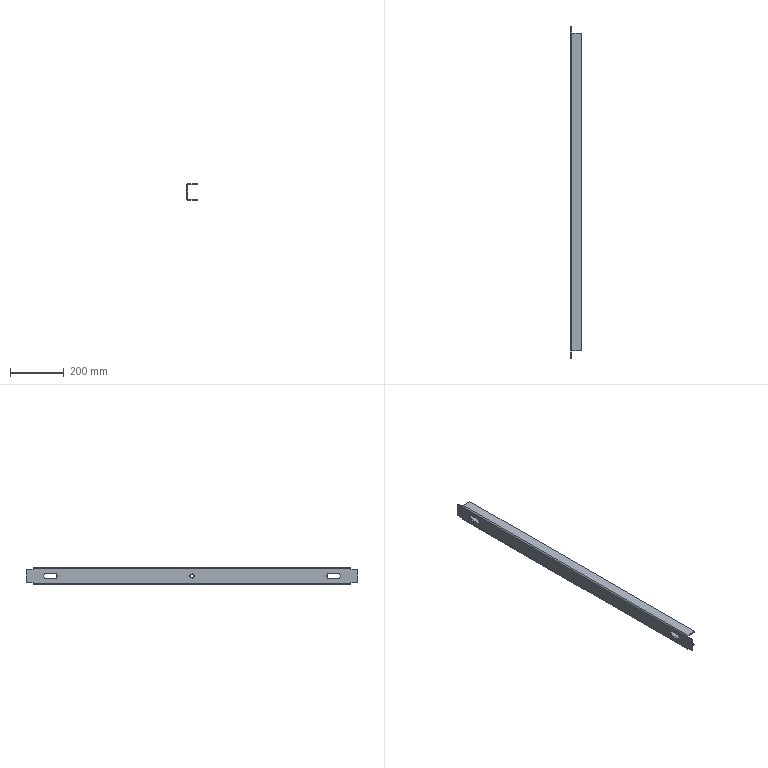Part | 1 solid | 44 faces | box 40 x 1230 x 62 mm | volume 624803 mm3 | plane 30 | cylinder 14 | commonest cylinder face diameters 10 x4 20 x4 0.4 x2 8.4 x2 15 x2
STEP:
#1=CARTESIAN_POINT('',(0.,0.,-7.5));
#2=VERTEX_POINT('',#1);
#3=CARTESIAN_POINT('',(0.,0.,7.5));
#4=VERTEX_POINT('',#3);
#5=CARTESIAN_POINT('',(0.,0.,0.));
#6=DIRECTION('',(-1.,0.,0.));
#7=DIRECTION('',(0.,0.,1.));
#8=AXIS2_PLACEMENT_3D('',#5,#6,#7);
#9=CIRCLE('',#8,7.5);
#10=EDGE_CURVE('',#2,#4,#9,.T.);
#11=ORIENTED_EDGE('',*,*,#10,.T.);
#12=CARTESIAN_POINT('',(4.,0.,7.5));
#13=VERTEX_POINT('',#12);
#14=CARTESIAN_POINT('',(-6.,0.,7.5));
#15=DIRECTION('',(1.,0.,0.));
#16=VECTOR('',#15,1000.);
#17=LINE('',#14,#16);
#18=EDGE_CURVE('',#4,#13,#17,.T.);
#19=ORIENTED_EDGE('',*,*,#18,.T.);
#20=CARTESIAN_POINT('',(4.,0.,-7.5));
#21=VERTEX_POINT('',#20);
#22=CARTESIAN_POINT('',(4.,0.,0.));
#23=DIRECTION('',(1.,0.,0.));
#24=DIRECTION('',(0.,0.,-1.));
#25=AXIS2_PLACEMENT_3D('',#22,#23,#24);
#26=CIRCLE('',#25,7.5);
#27=EDGE_CURVE('',#13,#21,#26,.T.);
#28=ORIENTED_EDGE('',*,*,#27,.T.);
#29=CARTESIAN_POINT('',(-6.,0.,-7.5));
#30=DIRECTION('',(1.,0.,0.));
#31=VECTOR('',#30,1000.);
#32=LINE('',#29,#31);
#33=EDGE_CURVE('',#2,#21,#32,.T.);
#34=ORIENTED_EDGE('',*,*,#33,.F.);
#35=EDGE_LOOP('',(#11,#19,#28,#34));
#36=FACE_OUTER_BOUND('',#35,.T.);
#37=CARTESIAN_POINT('',(-6.,0.,0.));
#38=DIRECTION('',(1.,0.,0.));
#39=DIRECTION('',(0.,0.,-1.));
#40=AXIS2_PLACEMENT_3D('',#37,#38,#39);
#41=CYLINDRICAL_SURFACE('',#40,7.5);
#42=ADVANCED_FACE('',(#36),#41,.F.);
#43=CARTESIAN_POINT('',(4.,-589.,25.));
#44=VERTEX_POINT('',#43);
#45=CARTESIAN_POINT('',(0.,-589.,25.));
#46=VERTEX_POINT('',#45);
#47=CARTESIAN_POINT('',(4.2,-589.,25.));
#48=DIRECTION('',(-1.,0.,0.));
#49=VECTOR('',#48,1000.);
#50=LINE('',#47,#49);
#51=EDGE_CURVE('',#44,#46,#50,.T.);
#52=ORIENTED_EDGE('',*,*,#51,.F.);
#53=CARTESIAN_POINT('',(4.,-589.,26.8));
#54=VERTEX_POINT('',#53);
#55=CARTESIAN_POINT('',(4.,-589.,-31.));
#56=DIRECTION('',(0.,0.,-1.));
#57=VECTOR('',#56,1000.);
#58=LINE('',#55,#57);
#59=EDGE_CURVE('',#54,#44,#58,.T.);
#60=ORIENTED_EDGE('',*,*,#59,.F.);
#61=CARTESIAN_POINT('',(0.,-589.,26.8));
#62=VERTEX_POINT('',#61);
#63=CARTESIAN_POINT('',(4.,-589.,26.8));
#64=DIRECTION('',(-1.,0.,0.));
#65=VECTOR('',#64,1000.);
#66=LINE('',#63,#65);
#67=EDGE_CURVE('',#54,#62,#66,.T.);
#68=ORIENTED_EDGE('',*,*,#67,.T.);
#69=CARTESIAN_POINT('',(0.,-589.,-31.));
#70=DIRECTION('',(0.,0.,-1.));
#71=VECTOR('',#70,1000.);
#72=LINE('',#69,#71);
#73=EDGE_CURVE('',#62,#46,#72,.T.);
#74=ORIENTED_EDGE('',*,*,#73,.T.);
#75=EDGE_LOOP('',(#52,#60,#68,#74));
#76=FACE_OUTER_BOUND('',#75,.T.);
#77=CARTESIAN_POINT('',(4.2,-589.,-27.));
#78=DIRECTION('',(0.,-1.,0.));
#79=DIRECTION('',(0.,0.,-1.));
#80=AXIS2_PLACEMENT_3D('',#77,#78,#79);
#81=PLANE('',#80);
#82=ADVANCED_FACE('',(#76),#81,.T.);
#83=CARTESIAN_POINT('',(4.,589.,-25.));
#84=VERTEX_POINT('',#83);
#85=CARTESIAN_POINT('',(0.,589.,-25.));
#86=VERTEX_POINT('',#85);
#87=CARTESIAN_POINT('',(4.2,589.,-25.));
#88=DIRECTION('',(-1.,0.,0.));
#89=VECTOR('',#88,1000.);
#90=LINE('',#87,#89);
#91=EDGE_CURVE('',#84,#86,#90,.T.);
#92=ORIENTED_EDGE('',*,*,#91,.F.);
#93=CARTESIAN_POINT('',(4.,589.,-26.8));
#94=VERTEX_POINT('',#93);
#95=CARTESIAN_POINT('',(4.,589.,-31.));
#96=DIRECTION('',(0.,0.,-1.));
#97=VECTOR('',#96,1000.);
#98=LINE('',#95,#97);
#99=EDGE_CURVE('',#84,#94,#98,.T.);
#100=ORIENTED_EDGE('',*,*,#99,.T.);
#101=CARTESIAN_POINT('',(0.,589.,-26.8));
#102=VERTEX_POINT('',#101);
#103=CARTESIAN_POINT('',(4.,589.,-26.8));
#104=DIRECTION('',(-1.,0.,0.));
#105=VECTOR('',#104,1000.);
#106=LINE('',#103,#105);
#107=EDGE_CURVE('',#94,#102,#106,.T.);
#108=ORIENTED_EDGE('',*,*,#107,.T.);
#109=CARTESIAN_POINT('',(0.,589.,-31.));
#110=DIRECTION('',(0.,0.,-1.));
#111=VECTOR('',#110,1000.);
#112=LINE('',#109,#111);
#113=EDGE_CURVE('',#86,#102,#112,.T.);
#114=ORIENTED_EDGE('',*,*,#113,.F.);
#115=EDGE_LOOP('',(#92,#100,#108,#114));
#116=FACE_OUTER_BOUND('',#115,.T.);
#117=CARTESIAN_POINT('',(4.2,589.,27.));
#118=DIRECTION('',(0.,1.,0.));
#119=DIRECTION('',(0.,0.,1.));
#120=AXIS2_PLACEMENT_3D('',#117,#118,#119);
#121=PLANE('',#120);
#122=ADVANCED_FACE('',(#116),#121,.T.);
#123=CARTESIAN_POINT('',(0.,589.,26.8));
#124=VERTEX_POINT('',#123);
#125=CARTESIAN_POINT('',(4.,589.,26.8));
#126=VERTEX_POINT('',#125);
#127=CARTESIAN_POINT('',(0.,589.,26.8));
#128=DIRECTION('',(1.,0.,0.));
#129=VECTOR('',#128,1000.);
#130=LINE('',#127,#129);
#131=EDGE_CURVE('',#124,#126,#130,.T.);
#132=ORIENTED_EDGE('',*,*,#131,.F.);
#133=CARTESIAN_POINT('',(4.2,589.,31.));
#134=VERTEX_POINT('',#133);
#135=CARTESIAN_POINT('',(4.2,589.,26.8));
#136=DIRECTION('',(0.,-1.,0.));
#137=DIRECTION('',(0.,0.,1.));
#138=AXIS2_PLACEMENT_3D('',#135,#136,#137);
#139=CIRCLE('',#138,4.2);
#140=EDGE_CURVE('',#134,#124,#139,.T.);
#141=ORIENTED_EDGE('',*,*,#140,.F.);
#142=CARTESIAN_POINT('',(4.2,589.,27.));
#143=VERTEX_POINT('',#142);
#144=CARTESIAN_POINT('',(4.2,589.,27.));
#145=DIRECTION('',(0.,0.,1.));
#146=VECTOR('',#145,1000.);
#147=LINE('',#144,#146);
#148=EDGE_CURVE('',#143,#134,#147,.T.);
#149=ORIENTED_EDGE('',*,*,#148,.F.);
#150=CARTESIAN_POINT('',(4.2,589.,26.8));
#151=DIRECTION('',(0.,-1.,0.));
#152=DIRECTION('',(1.,0.,0.));
#153=AXIS2_PLACEMENT_3D('',#150,#151,#152);
#154=CIRCLE('',#153,0.2);
#155=EDGE_CURVE('',#143,#126,#154,.T.);
#156=ORIENTED_EDGE('',*,*,#155,.T.);
#157=EDGE_LOOP('',(#132,#141,#149,#156));
#158=FACE_OUTER_BOUND('',#157,.T.);
#159=CARTESIAN_POINT('',(0.,589.,26.8));
#160=DIRECTION('',(0.,1.,0.));
#161=DIRECTION('',(0.,0.,1.));
#162=AXIS2_PLACEMENT_3D('',#159,#160,#161);
#163=PLANE('',#162);
#164=ADVANCED_FACE('',(#158),#163,.T.);
#165=CARTESIAN_POINT('',(0.,589.,25.));
#166=VERTEX_POINT('',#165);
#167=CARTESIAN_POINT('',(4.,589.,25.));
#168=VERTEX_POINT('',#167);
#169=CARTESIAN_POINT('',(4.2,589.,25.));
#170=DIRECTION('',(1.,0.,0.));
#171=VECTOR('',#170,1000.);
#172=LINE('',#169,#171);
#173=EDGE_CURVE('',#166,#168,#172,.T.);
#174=ORIENTED_EDGE('',*,*,#173,.F.);
#175=CARTESIAN_POINT('',(0.,589.,-31.));
#176=DIRECTION('',(0.,0.,-1.));
#177=VECTOR('',#176,1000.);
#178=LINE('',#175,#177);
#179=EDGE_CURVE('',#124,#166,#178,.T.);
#180=ORIENTED_EDGE('',*,*,#179,.F.);
#181=ORIENTED_EDGE('',*,*,#131,.T.);
#182=CARTESIAN_POINT('',(4.,589.,-31.));
#183=DIRECTION('',(0.,0.,-1.));
#184=VECTOR('',#183,1000.);
#185=LINE('',#182,#184);
#186=EDGE_CURVE('',#126,#168,#185,.T.);
#187=ORIENTED_EDGE('',*,*,#186,.T.);
#188=EDGE_LOOP('',(#174,#180,#181,#187));
#189=FACE_OUTER_BOUND('',#188,.T.);
#190=CARTESIAN_POINT('',(4.2,589.,27.));
#191=DIRECTION('',(0.,1.,0.));
#192=DIRECTION('',(0.,0.,1.));
#193=AXIS2_PLACEMENT_3D('',#190,#191,#192);
#194=PLANE('',#193);
#195=ADVANCED_FACE('',(#189),#194,.T.);
#196=CARTESIAN_POINT('',(4.2,-589.,31.));
#197=VERTEX_POINT('',#196);
#198=CARTESIAN_POINT('',(4.2,-589.,27.));
#199=VERTEX_POINT('',#198);
#200=CARTESIAN_POINT('',(4.2,-589.,31.));
#201=DIRECTION('',(0.,0.,-1.));
#202=VECTOR('',#201,1000.);
#203=LINE('',#200,#202);
#204=EDGE_CURVE('',#197,#199,#203,.T.);
#205=ORIENTED_EDGE('',*,*,#204,.F.);
#206=CARTESIAN_POINT('',(4.2,-589.,26.8));
#207=DIRECTION('',(0.,-1.,0.));
#208=DIRECTION('',(0.,0.,1.));
#209=AXIS2_PLACEMENT_3D('',#206,#207,#208);
#210=CIRCLE('',#209,4.2);
#211=EDGE_CURVE('',#197,#62,#210,.T.);
#212=ORIENTED_EDGE('',*,*,#211,.T.);
#213=ORIENTED_EDGE('',*,*,#67,.F.);
#214=CARTESIAN_POINT('',(4.2,-589.,26.8));
#215=DIRECTION('',(0.,-1.,0.));
#216=DIRECTION('',(1.,0.,0.));
#217=AXIS2_PLACEMENT_3D('',#214,#215,#216);
#218=CIRCLE('',#217,0.2);
#219=EDGE_CURVE('',#199,#54,#218,.T.);
#220=ORIENTED_EDGE('',*,*,#219,.F.);
#221=EDGE_LOOP('',(#205,#212,#213,#220));
#222=FACE_OUTER_BOUND('',#221,.T.);
#223=CARTESIAN_POINT('',(4.2,-589.,31.));
#224=DIRECTION('',(0.,-1.,0.));
#225=DIRECTION('',(0.,0.,-1.));
#226=AXIS2_PLACEMENT_3D('',#223,#224,#225);
#227=PLANE('',#226);
#228=ADVANCED_FACE('',(#222),#227,.T.);
#229=CARTESIAN_POINT('',(40.,-589.,31.));
#230=VERTEX_POINT('',#229);
#231=CARTESIAN_POINT('',(0.,-589.,31.));
#232=DIRECTION('',(-1.,0.,0.));
#233=VECTOR('',#232,1000.);
#234=LINE('',#231,#233);
#235=EDGE_CURVE('',#230,#197,#234,.T.);
#236=ORIENTED_EDGE('',*,*,#235,.T.);
#237=ORIENTED_EDGE('',*,*,#204,.T.);
#238=CARTESIAN_POINT('',(40.,-589.,27.));
#239=VERTEX_POINT('',#238);
#240=CARTESIAN_POINT('',(0.,-589.,27.));
#241=DIRECTION('',(-1.,0.,0.));
#242=VECTOR('',#241,1000.);
#243=LINE('',#240,#242);
#244=EDGE_CURVE('',#239,#199,#243,.T.);
#245=ORIENTED_EDGE('',*,*,#244,.F.);
#246=CARTESIAN_POINT('',(40.,-589.,27.));
#247=DIRECTION('',(0.,0.,1.));
#248=VECTOR('',#247,1000.);
#249=LINE('',#246,#248);
#250=EDGE_CURVE('',#239,#230,#249,.T.);
#251=ORIENTED_EDGE('',*,*,#250,.T.);
#252=EDGE_LOOP('',(#236,#237,#245,#251));
#253=FACE_OUTER_BOUND('',#252,.T.);
#254=CARTESIAN_POINT('',(4.,-589.,26.8));
#255=DIRECTION('',(0.,-1.,0.));
#256=DIRECTION('',(0.,0.,-1.));
#257=AXIS2_PLACEMENT_3D('',#254,#255,#256);
#258=PLANE('',#257);
#259=ADVANCED_FACE('',(#253),#258,.T.);
#260=CARTESIAN_POINT('',(4.2,589.,-31.));
#261=VERTEX_POINT('',#260);
#262=CARTESIAN_POINT('',(4.2,589.,-27.));
#263=VERTEX_POINT('',#262);
#264=CARTESIAN_POINT('',(4.2,589.,-31.));
#265=DIRECTION('',(0.,0.,1.));
#266=VECTOR('',#265,1000.);
#267=LINE('',#264,#266);
#268=EDGE_CURVE('',#261,#263,#267,.T.);
#269=ORIENTED_EDGE('',*,*,#268,.F.);
#270=CARTESIAN_POINT('',(4.2,589.,-26.8));
#271=DIRECTION('',(0.,-1.,0.));
#272=DIRECTION('',(0.,0.,1.));
#273=AXIS2_PLACEMENT_3D('',#270,#271,#272);
#274=CIRCLE('',#273,4.2);
#275=EDGE_CURVE('',#102,#261,#274,.T.);
#276=ORIENTED_EDGE('',*,*,#275,.F.);
#277=ORIENTED_EDGE('',*,*,#107,.F.);
#278=CARTESIAN_POINT('',(4.2,589.,-26.8));
#279=DIRECTION('',(0.,-1.,0.));
#280=DIRECTION('',(1.,0.,0.));
#281=AXIS2_PLACEMENT_3D('',#278,#279,#280);
#282=CIRCLE('',#281,0.2);
#283=EDGE_CURVE('',#94,#263,#282,.T.);
#284=ORIENTED_EDGE('',*,*,#283,.T.);
#285=EDGE_LOOP('',(#269,#276,#277,#284));
#286=FACE_OUTER_BOUND('',#285,.T.);
#287=CARTESIAN_POINT('',(4.2,589.,-31.));
#288=DIRECTION('',(0.,1.,0.));
#289=DIRECTION('',(0.,0.,1.));
#290=AXIS2_PLACEMENT_3D('',#287,#288,#289);
#291=PLANE('',#290);
#292=ADVANCED_FACE('',(#286),#291,.T.);
#293=CARTESIAN_POINT('',(40.,589.,-31.));
#294=VERTEX_POINT('',#293);
#295=CARTESIAN_POINT('',(0.,589.,-31.));
#296=DIRECTION('',(1.,0.,0.));
#297=VECTOR('',#296,1000.);
#298=LINE('',#295,#297);
#299=EDGE_CURVE('',#261,#294,#298,.T.);
#300=ORIENTED_EDGE('',*,*,#299,.F.);
#301=ORIENTED_EDGE('',*,*,#268,.T.);
#302=CARTESIAN_POINT('',(40.,589.,-27.));
#303=VERTEX_POINT('',#302);
#304=CARTESIAN_POINT('',(0.,589.,-27.));
#305=DIRECTION('',(1.,0.,0.));
#306=VECTOR('',#305,1000.);
#307=LINE('',#304,#306);
#308=EDGE_CURVE('',#263,#303,#307,.T.);
#309=ORIENTED_EDGE('',*,*,#308,.T.);
#310=CARTESIAN_POINT('',(40.,589.,-31.));
#311=DIRECTION('',(0.,0.,1.));
#312=VECTOR('',#311,1000.);
#313=LINE('',#310,#312);
#314=EDGE_CURVE('',#294,#303,#313,.T.);
#315=ORIENTED_EDGE('',*,*,#314,.F.);
#316=EDGE_LOOP('',(#300,#301,#309,#315));
#317=FACE_OUTER_BOUND('',#316,.T.);
#318=CARTESIAN_POINT('',(4.,589.,-26.8));
#319=DIRECTION('',(0.,1.,0.));
#320=DIRECTION('',(0.,0.,1.));
#321=AXIS2_PLACEMENT_3D('',#318,#319,#320);
#322=PLANE('',#321);
#323=ADVANCED_FACE('',(#317),#322,.T.);
#324=CARTESIAN_POINT('',(0.,-589.,-26.8));
#325=VERTEX_POINT('',#324);
#326=CARTESIAN_POINT('',(4.,-589.,-26.8));
#327=VERTEX_POINT('',#326);
#328=CARTESIAN_POINT('',(0.,-589.,-26.8));
#329=DIRECTION('',(1.,0.,0.));
#330=VECTOR('',#329,1000.);
#331=LINE('',#328,#330);
#332=EDGE_CURVE('',#325,#327,#331,.T.);
#333=ORIENTED_EDGE('',*,*,#332,.F.);
#334=CARTESIAN_POINT('',(4.2,-589.,-31.));
#335=VERTEX_POINT('',#334);
#336=CARTESIAN_POINT('',(4.2,-589.,-26.8));
#337=DIRECTION('',(0.,-1.,0.));
#338=DIRECTION('',(0.,0.,1.));
#339=AXIS2_PLACEMENT_3D('',#336,#337,#338);
#340=CIRCLE('',#339,4.2);
#341=EDGE_CURVE('',#325,#335,#340,.T.);
#342=ORIENTED_EDGE('',*,*,#341,.T.);
#343=CARTESIAN_POINT('',(4.2,-589.,-27.));
#344=VERTEX_POINT('',#343);
#345=CARTESIAN_POINT('',(4.2,-589.,-27.));
#346=DIRECTION('',(0.,0.,-1.));
#347=VECTOR('',#346,1000.);
#348=LINE('',#345,#347);
#349=EDGE_CURVE('',#344,#335,#348,.T.);
#350=ORIENTED_EDGE('',*,*,#349,.F.);
#351=CARTESIAN_POINT('',(4.2,-589.,-26.8));
#352=DIRECTION('',(0.,-1.,0.));
#353=DIRECTION('',(1.,0.,0.));
#354=AXIS2_PLACEMENT_3D('',#351,#352,#353);
#355=CIRCLE('',#354,0.2);
#356=EDGE_CURVE('',#327,#344,#355,.T.);
#357=ORIENTED_EDGE('',*,*,#356,.F.);
#358=EDGE_LOOP('',(#333,#342,#350,#357));
#359=FACE_OUTER_BOUND('',#358,.T.);
#360=CARTESIAN_POINT('',(0.,-589.,-26.8));
#361=DIRECTION('',(0.,-1.,0.));
#362=DIRECTION('',(0.,0.,-1.));
#363=AXIS2_PLACEMENT_3D('',#360,#361,#362);
#364=PLANE('',#363);
#365=ADVANCED_FACE('',(#359),#364,.T.);
#366=CARTESIAN_POINT('',(0.,-589.,-25.));
#367=VERTEX_POINT('',#366);
#368=CARTESIAN_POINT('',(4.,-589.,-25.));
#369=VERTEX_POINT('',#368);
#370=CARTESIAN_POINT('',(4.2,-589.,-25.));
#371=DIRECTION('',(1.,0.,0.));
#372=VECTOR('',#371,1000.);
#373=LINE('',#370,#372);
#374=EDGE_CURVE('',#367,#369,#373,.T.);
#375=ORIENTED_EDGE('',*,*,#374,.F.);
#376=CARTESIAN_POINT('',(0.,-589.,-31.));
#377=DIRECTION('',(0.,0.,-1.));
#378=VECTOR('',#377,1000.);
#379=LINE('',#376,#378);
#380=EDGE_CURVE('',#367,#325,#379,.T.);
#381=ORIENTED_EDGE('',*,*,#380,.T.);
#382=ORIENTED_EDGE('',*,*,#332,.T.);
#383=CARTESIAN_POINT('',(4.,-589.,-31.));
#384=DIRECTION('',(0.,0.,-1.));
#385=VECTOR('',#384,1000.);
#386=LINE('',#383,#385);
#387=EDGE_CURVE('',#369,#327,#386,.T.);
#388=ORIENTED_EDGE('',*,*,#387,.F.);
#389=EDGE_LOOP('',(#375,#381,#382,#388));
#390=FACE_OUTER_BOUND('',#389,.T.);
#391=CARTESIAN_POINT('',(4.2,-589.,-27.));
#392=DIRECTION('',(0.,-1.,0.));
#393=DIRECTION('',(0.,0.,-1.));
#394=AXIS2_PLACEMENT_3D('',#391,#392,#393);
#395=PLANE('',#394);
#396=ADVANCED_FACE('',(#390),#395,.T.);
#397=CARTESIAN_POINT('',(40.,-589.,-27.));
#398=VERTEX_POINT('',#397);
#399=CARTESIAN_POINT('',(0.,-589.,-27.));
#400=DIRECTION('',(1.,0.,0.));
#401=VECTOR('',#400,1000.);
#402=LINE('',#399,#401);
#403=EDGE_CURVE('',#344,#398,#402,.T.);
#404=ORIENTED_EDGE('',*,*,#403,.T.);
#405=CARTESIAN_POINT('',(40.,589.,-27.));
#406=DIRECTION('',(0.,-1.,0.));
#407=VECTOR('',#406,1000.);
#408=LINE('',#405,#407);
#409=EDGE_CURVE('',#303,#398,#408,.T.);
#410=ORIENTED_EDGE('',*,*,#409,.F.);
#411=ORIENTED_EDGE('',*,*,#308,.F.);
#412=CARTESIAN_POINT('',(4.2,589.,-27.));
#413=DIRECTION('',(0.,-1.,0.));
#414=VECTOR('',#413,1000.);
#415=LINE('',#412,#414);
#416=EDGE_CURVE('',#263,#344,#415,.T.);
#417=ORIENTED_EDGE('',*,*,#416,.T.);
#418=EDGE_LOOP('',(#404,#410,#411,#417));
#419=FACE_OUTER_BOUND('',#418,.T.);
#420=CARTESIAN_POINT('',(0.,589.,-27.));
#421=DIRECTION('',(0.,0.,-1.));
#422=DIRECTION('',(-1.,0.,0.));
#423=AXIS2_PLACEMENT_3D('',#420,#421,#422);
#424=PLANE('',#423);
#425=ADVANCED_FACE('',(#419),#424,.F.);
#426=CARTESIAN_POINT('',(40.,-589.,-31.));
#427=VERTEX_POINT('',#426);
#428=CARTESIAN_POINT('',(40.,-589.,-31.));
#429=DIRECTION('',(0.,0.,1.));
#430=VECTOR('',#429,1000.);
#431=LINE('',#428,#430);
#432=EDGE_CURVE('',#427,#398,#431,.T.);
#433=ORIENTED_EDGE('',*,*,#432,.F.);
#434=CARTESIAN_POINT('',(40.,589.,-31.));
#435=DIRECTION('',(0.,-1.,0.));
#436=VECTOR('',#435,1000.);
#437=LINE('',#434,#436);
#438=EDGE_CURVE('',#294,#427,#437,.T.);
#439=ORIENTED_EDGE('',*,*,#438,.F.);
#440=ORIENTED_EDGE('',*,*,#314,.T.);
#441=ORIENTED_EDGE('',*,*,#409,.T.);
#442=EDGE_LOOP('',(#433,#439,#440,#441));
#443=FACE_OUTER_BOUND('',#442,.T.);
#444=CARTESIAN_POINT('',(40.,589.,-31.));
#445=DIRECTION('',(1.,0.,0.));
#446=DIRECTION('',(0.,0.,-1.));
#447=AXIS2_PLACEMENT_3D('',#444,#445,#446);
#448=PLANE('',#447);
#449=ADVANCED_FACE('',(#443),#448,.T.);
#450=CARTESIAN_POINT('',(0.,-589.,-31.));
#451=DIRECTION('',(1.,0.,0.));
#452=VECTOR('',#451,1000.);
#453=LINE('',#450,#452);
#454=EDGE_CURVE('',#335,#427,#453,.T.);
#455=ORIENTED_EDGE('',*,*,#454,.F.);
#456=CARTESIAN_POINT('',(4.2,589.,-31.));
#457=DIRECTION('',(0.,-1.,0.));
#458=VECTOR('',#457,1000.);
#459=LINE('',#456,#458);
#460=EDGE_CURVE('',#261,#335,#459,.T.);
#461=ORIENTED_EDGE('',*,*,#460,.F.);
#462=ORIENTED_EDGE('',*,*,#299,.T.);
#463=ORIENTED_EDGE('',*,*,#438,.T.);
#464=EDGE_LOOP('',(#455,#461,#462,#463));
#465=FACE_OUTER_BOUND('',#464,.T.);
#466=CARTESIAN_POINT('',(0.,589.,-31.));
#467=DIRECTION('',(0.,0.,-1.));
#468=DIRECTION('',(-1.,0.,0.));
#469=AXIS2_PLACEMENT_3D('',#466,#467,#468);
#470=PLANE('',#469);
#471=ADVANCED_FACE('',(#465),#470,.T.);
#472=ORIENTED_EDGE('',*,*,#341,.F.);
#473=CARTESIAN_POINT('',(0.,589.,-26.8));
#474=DIRECTION('',(0.,-1.,0.));
#475=VECTOR('',#474,1000.);
#476=LINE('',#473,#475);
#477=EDGE_CURVE('',#102,#325,#476,.T.);
#478=ORIENTED_EDGE('',*,*,#477,.F.);
#479=ORIENTED_EDGE('',*,*,#275,.T.);
#480=ORIENTED_EDGE('',*,*,#460,.T.);
#481=EDGE_LOOP('',(#472,#478,#479,#480));
#482=FACE_OUTER_BOUND('',#481,.T.);
#483=CARTESIAN_POINT('',(4.2,589.,-26.8));
#484=DIRECTION('',(0.,-1.,0.));
#485=DIRECTION('',(0.,0.,-1.));
#486=AXIS2_PLACEMENT_3D('',#483,#484,#485);
#487=CYLINDRICAL_SURFACE('',#486,4.2);
#488=ADVANCED_FACE('',(#482),#487,.T.);
#489=CARTESIAN_POINT('',(0.,510.,-10.));
#490=VERTEX_POINT('',#489);
#491=CARTESIAN_POINT('',(0.,510.,10.));
#492=VERTEX_POINT('',#491);
#493=CARTESIAN_POINT('',(0.,510.,0.));
#494=DIRECTION('',(-1.,0.,0.));
#495=DIRECTION('',(0.,0.,1.));
#496=AXIS2_PLACEMENT_3D('',#493,#494,#495);
#497=CIRCLE('',#496,10.);
#498=EDGE_CURVE('',#490,#492,#497,.T.);
#499=ORIENTED_EDGE('',*,*,#498,.F.);
#500=CARTESIAN_POINT('',(0.,540.,-10.));
#501=VERTEX_POINT('',#500);
#502=CARTESIAN_POINT('',(0.,589.,-10.));
#503=DIRECTION('',(0.,-1.,0.));
#504=VECTOR('',#503,1000.);
#505=LINE('',#502,#504);
#506=EDGE_CURVE('',#501,#490,#505,.T.);
#507=ORIENTED_EDGE('',*,*,#506,.F.);
#508=CARTESIAN_POINT('',(0.,540.,10.));
#509=VERTEX_POINT('',#508);
#510=CARTESIAN_POINT('',(0.,540.,0.));
#511=DIRECTION('',(-1.,0.,0.));
#512=DIRECTION('',(0.,0.,1.));
#513=AXIS2_PLACEMENT_3D('',#510,#511,#512);
#514=CIRCLE('',#513,10.);
#515=EDGE_CURVE('',#509,#501,#514,.T.);
#516=ORIENTED_EDGE('',*,*,#515,.F.);
#517=CARTESIAN_POINT('',(0.,589.,10.));
#518=DIRECTION('',(0.,1.,0.));
#519=VECTOR('',#518,1000.);
#520=LINE('',#517,#519);
#521=EDGE_CURVE('',#492,#509,#520,.T.);
#522=ORIENTED_EDGE('',*,*,#521,.F.);
#523=EDGE_LOOP('',(#499,#507,#516,#522));
#524=FACE_BOUND('',#523,.T.);
#525=ORIENTED_EDGE('',*,*,#10,.F.);
#526=CARTESIAN_POINT('',(0.,0.,0.));
#527=DIRECTION('',(-1.,0.,0.));
#528=DIRECTION('',(0.,0.,1.));
#529=AXIS2_PLACEMENT_3D('',#526,#527,#528);
#530=CIRCLE('',#529,7.5);
#531=EDGE_CURVE('',#4,#2,#530,.T.);
#532=ORIENTED_EDGE('',*,*,#531,.F.);
#533=EDGE_LOOP('',(#525,#532));
#534=FACE_BOUND('',#533,.T.);
#535=CARTESIAN_POINT('',(0.,-510.,10.));
#536=VERTEX_POINT('',#535);
#537=CARTESIAN_POINT('',(0.,-510.,-10.));
#538=VERTEX_POINT('',#537);
#539=CARTESIAN_POINT('',(0.,-510.,0.));
#540=DIRECTION('',(-1.,0.,0.));
#541=DIRECTION('',(0.,0.,1.));
#542=AXIS2_PLACEMENT_3D('',#539,#540,#541);
#543=CIRCLE('',#542,10.);
#544=EDGE_CURVE('',#536,#538,#543,.T.);
#545=ORIENTED_EDGE('',*,*,#544,.F.);
#546=CARTESIAN_POINT('',(0.,-540.,10.));
#547=VERTEX_POINT('',#546);
#548=CARTESIAN_POINT('',(0.,589.,10.));
#549=DIRECTION('',(0.,1.,0.));
#550=VECTOR('',#549,1000.);
#551=LINE('',#548,#550);
#552=EDGE_CURVE('',#547,#536,#551,.T.);
#553=ORIENTED_EDGE('',*,*,#552,.F.);
#554=CARTESIAN_POINT('',(0.,-540.,-10.));
#555=VERTEX_POINT('',#554);
#556=CARTESIAN_POINT('',(0.,-540.,0.));
#557=DIRECTION('',(-1.,0.,0.));
#558=DIRECTION('',(0.,0.,1.));
#559=AXIS2_PLACEMENT_3D('',#556,#557,#558);
#560=CIRCLE('',#559,10.);
#561=EDGE_CURVE('',#555,#547,#560,.T.);
#562=ORIENTED_EDGE('',*,*,#561,.F.);
#563=CARTESIAN_POINT('',(0.,589.,-10.));
#564=DIRECTION('',(0.,-1.,0.));
#565=VECTOR('',#564,1000.);
#566=LINE('',#563,#565);
#567=EDGE_CURVE('',#538,#555,#566,.T.);
#568=ORIENTED_EDGE('',*,*,#567,.F.);
#569=EDGE_LOOP('',(#545,#553,#562,#568));
#570=FACE_BOUND('',#569,.T.);
#571=CARTESIAN_POINT('',(0.,-610.,-25.));
#572=VERTEX_POINT('',#571);
#573=CARTESIAN_POINT('',(0.,-615.,-25.));
#574=DIRECTION('',(0.,1.,0.));
#575=VECTOR('',#574,1000.);
#576=LINE('',#573,#575);
#577=EDGE_CURVE('',#572,#367,#576,.T.);
#578=ORIENTED_EDGE('',*,*,#577,.F.);
#579=CARTESIAN_POINT('',(0.,-615.,-20.));
#580=VERTEX_POINT('',#579);
#581=CARTESIAN_POINT('',(0.,-610.,-20.));
#582=DIRECTION('',(-1.,0.,0.));
#583=DIRECTION('',(0.,0.,1.));
#584=AXIS2_PLACEMENT_3D('',#581,#582,#583);
#585=CIRCLE('',#584,5.);
#586=EDGE_CURVE('',#572,#580,#585,.T.);
#587=ORIENTED_EDGE('',*,*,#586,.T.);
#588=CARTESIAN_POINT('',(0.,-615.,20.));
#589=VERTEX_POINT('',#588);
#590=CARTESIAN_POINT('',(0.,-615.,25.));
#591=DIRECTION('',(0.,0.,-1.));
#592=VECTOR('',#591,1000.);
#593=LINE('',#590,#592);
#594=EDGE_CURVE('',#589,#580,#593,.T.);
#595=ORIENTED_EDGE('',*,*,#594,.F.);
#596=CARTESIAN_POINT('',(0.,-610.,25.));
#597=VERTEX_POINT('',#596);
#598=CARTESIAN_POINT('',(0.,-610.,20.));
#599=DIRECTION('',(-1.,0.,0.));
#600=DIRECTION('',(0.,0.,1.));
#601=AXIS2_PLACEMENT_3D('',#598,#599,#600);
#602=CIRCLE('',#601,5.);
#603=EDGE_CURVE('',#589,#597,#602,.T.);
#604=ORIENTED_EDGE('',*,*,#603,.T.);
#605=CARTESIAN_POINT('',(0.,-615.,25.));
#606=DIRECTION('',(0.,-1.,0.));
#607=VECTOR('',#606,1000.);
#608=LINE('',#605,#607);
#609=EDGE_CURVE('',#46,#597,#608,.T.);
#610=ORIENTED_EDGE('',*,*,#609,.F.);
#611=ORIENTED_EDGE('',*,*,#73,.F.);
#612=CARTESIAN_POINT('',(0.,589.,26.8));
#613=DIRECTION('',(0.,-1.,0.));
#614=VECTOR('',#613,1000.);
#615=LINE('',#612,#614);
#616=EDGE_CURVE('',#124,#62,#615,.T.);
#617=ORIENTED_EDGE('',*,*,#616,.F.);
#618=ORIENTED_EDGE('',*,*,#179,.T.);
#619=CARTESIAN_POINT('',(0.,610.,25.));
#620=VERTEX_POINT('',#619);
#621=CARTESIAN_POINT('',(0.,615.,25.));
#622=DIRECTION('',(0.,-1.,0.));
#623=VECTOR('',#622,1000.);
#624=LINE('',#621,#623);
#625=EDGE_CURVE('',#620,#166,#624,.T.);
#626=ORIENTED_EDGE('',*,*,#625,.F.);
#627=CARTESIAN_POINT('',(0.,615.,20.));
#628=VERTEX_POINT('',#627);
#629=CARTESIAN_POINT('',(0.,610.,20.));
#630=DIRECTION('',(-1.,0.,0.));
#631=DIRECTION('',(0.,0.,1.));
#632=AXIS2_PLACEMENT_3D('',#629,#630,#631);
#633=CIRCLE('',#632,5.);
#634=EDGE_CURVE('',#620,#628,#633,.T.);
#635=ORIENTED_EDGE('',*,*,#634,.T.);
#636=CARTESIAN_POINT('',(0.,615.,-20.));
#637=VERTEX_POINT('',#636);
#638=CARTESIAN_POINT('',(0.,615.,25.));
#639=DIRECTION('',(0.,0.,1.));
#640=VECTOR('',#639,1000.);
#641=LINE('',#638,#640);
#642=EDGE_CURVE('',#637,#628,#641,.T.);
#643=ORIENTED_EDGE('',*,*,#642,.F.);
#644=CARTESIAN_POINT('',(0.,610.,-25.));
#645=VERTEX_POINT('',#644);
#646=CARTESIAN_POINT('',(0.,610.,-20.));
#647=DIRECTION('',(-1.,0.,0.));
#648=DIRECTION('',(0.,0.,1.));
#649=AXIS2_PLACEMENT_3D('',#646,#647,#648);
#650=CIRCLE('',#649,5.);
#651=EDGE_CURVE('',#637,#645,#650,.T.);
#652=ORIENTED_EDGE('',*,*,#651,.T.);
#653=CARTESIAN_POINT('',(0.,615.,-25.));
#654=DIRECTION('',(0.,1.,0.));
#655=VECTOR('',#654,1000.);
#656=LINE('',#653,#655);
#657=EDGE_CURVE('',#86,#645,#656,.T.);
#658=ORIENTED_EDGE('',*,*,#657,.F.);
#659=ORIENTED_EDGE('',*,*,#113,.T.);
#660=ORIENTED_EDGE('',*,*,#477,.T.);
#661=ORIENTED_EDGE('',*,*,#380,.F.);
#662=EDGE_LOOP('',(#578,#587,#595,#604,#610,#611,#617,#618,#626,#635,#643,#652,#658,#659,#660,#661));
#663=FACE_OUTER_BOUND('',#662,.T.);
#664=CARTESIAN_POINT('',(0.,589.,-31.));
#665=DIRECTION('',(-1.,0.,0.));
#666=DIRECTION('',(0.,0.,1.));
#667=AXIS2_PLACEMENT_3D('',#664,#665,#666);
#668=PLANE('',#667);
#669=ADVANCED_FACE('',(#524,#534,#570,#663),#668,.T.);
#670=ORIENTED_EDGE('',*,*,#211,.F.);
#671=CARTESIAN_POINT('',(4.2,589.,31.));
#672=DIRECTION('',(0.,-1.,0.));
#673=VECTOR('',#672,1000.);
#674=LINE('',#671,#673);
#675=EDGE_CURVE('',#134,#197,#674,.T.);
#676=ORIENTED_EDGE('',*,*,#675,.F.);
#677=ORIENTED_EDGE('',*,*,#140,.T.);
#678=ORIENTED_EDGE('',*,*,#616,.T.);
#679=EDGE_LOOP('',(#670,#676,#677,#678));
#680=FACE_OUTER_BOUND('',#679,.T.);
#681=CARTESIAN_POINT('',(4.2,589.,26.8));
#682=DIRECTION('',(0.,-1.,0.));
#683=DIRECTION('',(0.,0.,-1.));
#684=AXIS2_PLACEMENT_3D('',#681,#682,#683);
#685=CYLINDRICAL_SURFACE('',#684,4.2);
#686=ADVANCED_FACE('',(#680),#685,.T.);
#687=ORIENTED_EDGE('',*,*,#235,.F.);
#688=CARTESIAN_POINT('',(40.,589.,31.));
#689=VERTEX_POINT('',#688);
#690=CARTESIAN_POINT('',(40.,589.,31.));
#691=DIRECTION('',(0.,-1.,0.));
#692=VECTOR('',#691,1000.);
#693=LINE('',#690,#692);
#694=EDGE_CURVE('',#689,#230,#693,.T.);
#695=ORIENTED_EDGE('',*,*,#694,.F.);
#696=CARTESIAN_POINT('',(0.,589.,31.));
#697=DIRECTION('',(-1.,0.,0.));
#698=VECTOR('',#697,1000.);
#699=LINE('',#696,#698);
#700=EDGE_CURVE('',#689,#134,#699,.T.);
#701=ORIENTED_EDGE('',*,*,#700,.T.);
#702=ORIENTED_EDGE('',*,*,#675,.T.);
#703=EDGE_LOOP('',(#687,#695,#701,#702));
#704=FACE_OUTER_BOUND('',#703,.T.);
#705=CARTESIAN_POINT('',(0.,589.,31.));
#706=DIRECTION('',(0.,0.,1.));
#707=DIRECTION('',(1.,0.,0.));
#708=AXIS2_PLACEMENT_3D('',#705,#706,#707);
#709=PLANE('',#708);
#710=ADVANCED_FACE('',(#704),#709,.T.);
#711=ORIENTED_EDGE('',*,*,#250,.F.);
#712=CARTESIAN_POINT('',(40.,589.,27.));
#713=VERTEX_POINT('',#712);
#714=CARTESIAN_POINT('',(40.,589.,27.));
#715=DIRECTION('',(0.,-1.,0.));
#716=VECTOR('',#715,1000.);
#717=LINE('',#714,#716);
#718=EDGE_CURVE('',#713,#239,#717,.T.);
#719=ORIENTED_EDGE('',*,*,#718,.F.);
#720=CARTESIAN_POINT('',(40.,589.,27.));
#721=DIRECTION('',(0.,0.,1.));
#722=VECTOR('',#721,1000.);
#723=LINE('',#720,#722);
#724=EDGE_CURVE('',#713,#689,#723,.T.);
#725=ORIENTED_EDGE('',*,*,#724,.T.);
#726=ORIENTED_EDGE('',*,*,#694,.T.);
#727=EDGE_LOOP('',(#711,#719,#725,#726));
#728=FACE_OUTER_BOUND('',#727,.T.);
#729=CARTESIAN_POINT('',(40.,589.,27.));
#730=DIRECTION('',(1.,0.,0.));
#731=DIRECTION('',(0.,0.,-1.));
#732=AXIS2_PLACEMENT_3D('',#729,#730,#731);
#733=PLANE('',#732);
#734=ADVANCED_FACE('',(#728),#733,.T.);
#735=ORIENTED_EDGE('',*,*,#244,.T.);
#736=CARTESIAN_POINT('',(4.2,589.,27.));
#737=DIRECTION('',(0.,-1.,0.));
#738=VECTOR('',#737,1000.);
#739=LINE('',#736,#738);
#740=EDGE_CURVE('',#143,#199,#739,.T.);
#741=ORIENTED_EDGE('',*,*,#740,.F.);
#742=CARTESIAN_POINT('',(0.,589.,27.));
#743=DIRECTION('',(-1.,0.,0.));
#744=VECTOR('',#743,1000.);
#745=LINE('',#742,#744);
#746=EDGE_CURVE('',#713,#143,#745,.T.);
#747=ORIENTED_EDGE('',*,*,#746,.F.);
#748=ORIENTED_EDGE('',*,*,#718,.T.);
#749=EDGE_LOOP('',(#735,#741,#747,#748));
#750=FACE_OUTER_BOUND('',#749,.T.);
#751=CARTESIAN_POINT('',(0.,589.,27.));
#752=DIRECTION('',(0.,0.,1.));
#753=DIRECTION('',(1.,0.,0.));
#754=AXIS2_PLACEMENT_3D('',#751,#752,#753);
#755=PLANE('',#754);
#756=ADVANCED_FACE('',(#750),#755,.F.);
#757=ORIENTED_EDGE('',*,*,#219,.T.);
#758=CARTESIAN_POINT('',(4.,589.,26.8));
#759=DIRECTION('',(0.,-1.,0.));
#760=VECTOR('',#759,1000.);
#761=LINE('',#758,#760);
#762=EDGE_CURVE('',#126,#54,#761,.T.);
#763=ORIENTED_EDGE('',*,*,#762,.F.);
#764=ORIENTED_EDGE('',*,*,#155,.F.);
#765=ORIENTED_EDGE('',*,*,#740,.T.);
#766=EDGE_LOOP('',(#757,#763,#764,#765));
#767=FACE_OUTER_BOUND('',#766,.T.);
#768=CARTESIAN_POINT('',(4.2,589.,26.8));
#769=DIRECTION('',(0.,-1.,0.));
#770=DIRECTION('',(0.,0.,-1.));
#771=AXIS2_PLACEMENT_3D('',#768,#769,#770);
#772=CYLINDRICAL_SURFACE('',#771,0.2);
#773=ADVANCED_FACE('',(#767),#772,.F.);
#774=CARTESIAN_POINT('',(4.,510.,-10.));
#775=VERTEX_POINT('',#774);
#776=CARTESIAN_POINT('',(4.,540.,-10.));
#777=VERTEX_POINT('',#776);
#778=CARTESIAN_POINT('',(4.,510.,-10.));
#779=DIRECTION('',(0.,1.,0.));
#780=VECTOR('',#779,1000.);
#781=LINE('',#778,#780);
#782=EDGE_CURVE('',#775,#777,#781,.T.);
#783=ORIENTED_EDGE('',*,*,#782,.F.);
#784=CARTESIAN_POINT('',(4.,510.,10.));
#785=VERTEX_POINT('',#784);
#786=CARTESIAN_POINT('',(4.,510.,0.));
#787=DIRECTION('',(1.,0.,0.));
#788=DIRECTION('',(0.,0.,-1.));
#789=AXIS2_PLACEMENT_3D('',#786,#787,#788);
#790=CIRCLE('',#789,10.);
#791=EDGE_CURVE('',#785,#775,#790,.T.);
#792=ORIENTED_EDGE('',*,*,#791,.F.);
#793=CARTESIAN_POINT('',(4.,540.,10.));
#794=VERTEX_POINT('',#793);
#795=CARTESIAN_POINT('',(4.,510.,10.));
#796=DIRECTION('',(0.,-1.,0.));
#797=VECTOR('',#796,1000.);
#798=LINE('',#795,#797);
#799=EDGE_CURVE('',#794,#785,#798,.T.);
#800=ORIENTED_EDGE('',*,*,#799,.F.);
#801=CARTESIAN_POINT('',(4.,540.,0.));
#802=DIRECTION('',(1.,0.,0.));
#803=DIRECTION('',(0.,0.,-1.));
#804=AXIS2_PLACEMENT_3D('',#801,#802,#803);
#805=CIRCLE('',#804,10.);
#806=EDGE_CURVE('',#777,#794,#805,.T.);
#807=ORIENTED_EDGE('',*,*,#806,.F.);
#808=EDGE_LOOP('',(#783,#792,#800,#807));
#809=FACE_BOUND('',#808,.T.);
#810=CARTESIAN_POINT('',(4.,0.,0.));
#811=DIRECTION('',(1.,0.,0.));
#812=DIRECTION('',(0.,0.,-1.));
#813=AXIS2_PLACEMENT_3D('',#810,#811,#812);
#814=CIRCLE('',#813,7.5);
#815=EDGE_CURVE('',#21,#13,#814,.T.);
#816=ORIENTED_EDGE('',*,*,#815,.F.);
#817=ORIENTED_EDGE('',*,*,#27,.F.);
#818=EDGE_LOOP('',(#816,#817));
#819=FACE_BOUND('',#818,.T.);
#820=CARTESIAN_POINT('',(4.,-510.,10.));
#821=VERTEX_POINT('',#820);
#822=CARTESIAN_POINT('',(4.,-540.,10.));
#823=VERTEX_POINT('',#822);
#824=CARTESIAN_POINT('',(4.,-510.,10.));
#825=DIRECTION('',(0.,-1.,0.));
#826=VECTOR('',#825,1000.);
#827=LINE('',#824,#826);
#828=EDGE_CURVE('',#821,#823,#827,.T.);
#829=ORIENTED_EDGE('',*,*,#828,.F.);
#830=CARTESIAN_POINT('',(4.,-510.,-10.));
#831=VERTEX_POINT('',#830);
#832=CARTESIAN_POINT('',(4.,-510.,0.));
#833=DIRECTION('',(1.,0.,0.));
#834=DIRECTION('',(0.,0.,1.));
#835=AXIS2_PLACEMENT_3D('',#832,#833,#834);
#836=CIRCLE('',#835,10.);
#837=EDGE_CURVE('',#831,#821,#836,.T.);
#838=ORIENTED_EDGE('',*,*,#837,.F.);
#839=CARTESIAN_POINT('',(4.,-540.,-10.));
#840=VERTEX_POINT('',#839);
#841=CARTESIAN_POINT('',(4.,-510.,-10.));
#842=DIRECTION('',(0.,1.,0.));
#843=VECTOR('',#842,1000.);
#844=LINE('',#841,#843);
#845=EDGE_CURVE('',#840,#831,#844,.T.);
#846=ORIENTED_EDGE('',*,*,#845,.F.);
#847=CARTESIAN_POINT('',(4.,-540.,0.));
#848=DIRECTION('',(1.,0.,0.));
#849=DIRECTION('',(0.,0.,1.));
#850=AXIS2_PLACEMENT_3D('',#847,#848,#849);
#851=CIRCLE('',#850,10.);
#852=EDGE_CURVE('',#823,#840,#851,.T.);
#853=ORIENTED_EDGE('',*,*,#852,.F.);
#854=EDGE_LOOP('',(#829,#838,#846,#853));
#855=FACE_BOUND('',#854,.T.);
#856=CARTESIAN_POINT('',(4.,-615.,20.));
#857=VERTEX_POINT('',#856);
#858=CARTESIAN_POINT('',(4.,-615.,-20.));
#859=VERTEX_POINT('',#858);
#860=CARTESIAN_POINT('',(4.,-615.,25.));
#861=DIRECTION('',(0.,0.,-1.));
#862=VECTOR('',#861,1000.);
#863=LINE('',#860,#862);
#864=EDGE_CURVE('',#857,#859,#863,.T.);
#865=ORIENTED_EDGE('',*,*,#864,.T.);
#866=CARTESIAN_POINT('',(4.,-610.,-25.));
#867=VERTEX_POINT('',#866);
#868=CARTESIAN_POINT('',(4.,-610.,-20.));
#869=DIRECTION('',(1.,0.,0.));
#870=DIRECTION('',(0.,0.,1.));
#871=AXIS2_PLACEMENT_3D('',#868,#869,#870);
#872=CIRCLE('',#871,5.);
#873=EDGE_CURVE('',#859,#867,#872,.T.);
#874=ORIENTED_EDGE('',*,*,#873,.T.);
#875=CARTESIAN_POINT('',(4.,-615.,-25.));
#876=DIRECTION('',(0.,1.,0.));
#877=VECTOR('',#876,1000.);
#878=LINE('',#875,#877);
#879=EDGE_CURVE('',#867,#369,#878,.T.);
#880=ORIENTED_EDGE('',*,*,#879,.T.);
#881=ORIENTED_EDGE('',*,*,#387,.T.);
#882=CARTESIAN_POINT('',(4.,589.,-26.8));
#883=DIRECTION('',(0.,-1.,0.));
#884=VECTOR('',#883,1000.);
#885=LINE('',#882,#884);
#886=EDGE_CURVE('',#94,#327,#885,.T.);
#887=ORIENTED_EDGE('',*,*,#886,.F.);
#888=ORIENTED_EDGE('',*,*,#99,.F.);
#889=CARTESIAN_POINT('',(4.,610.,-25.));
#890=VERTEX_POINT('',#889);
#891=CARTESIAN_POINT('',(4.,615.,-25.));
#892=DIRECTION('',(0.,1.,0.));
#893=VECTOR('',#892,1000.);
#894=LINE('',#891,#893);
#895=EDGE_CURVE('',#84,#890,#894,.T.);
#896=ORIENTED_EDGE('',*,*,#895,.T.);
#897=CARTESIAN_POINT('',(4.,615.,-20.));
#898=VERTEX_POINT('',#897);
#899=CARTESIAN_POINT('',(4.,610.,-20.));
#900=DIRECTION('',(1.,0.,0.));
#901=DIRECTION('',(0.,0.,1.));
#902=AXIS2_PLACEMENT_3D('',#899,#900,#901);
#903=CIRCLE('',#902,5.);
#904=EDGE_CURVE('',#890,#898,#903,.T.);
#905=ORIENTED_EDGE('',*,*,#904,.T.);
#906=CARTESIAN_POINT('',(4.,615.,20.));
#907=VERTEX_POINT('',#906);
#908=CARTESIAN_POINT('',(4.,615.,25.));
#909=DIRECTION('',(0.,0.,1.));
#910=VECTOR('',#909,1000.);
#911=LINE('',#908,#910);
#912=EDGE_CURVE('',#898,#907,#911,.T.);
#913=ORIENTED_EDGE('',*,*,#912,.T.);
#914=CARTESIAN_POINT('',(4.,610.,25.));
#915=VERTEX_POINT('',#914);
#916=CARTESIAN_POINT('',(4.,610.,20.));
#917=DIRECTION('',(1.,0.,0.));
#918=DIRECTION('',(0.,0.,1.));
#919=AXIS2_PLACEMENT_3D('',#916,#917,#918);
#920=CIRCLE('',#919,5.);
#921=EDGE_CURVE('',#907,#915,#920,.T.);
#922=ORIENTED_EDGE('',*,*,#921,.T.);
#923=CARTESIAN_POINT('',(4.,615.,25.));
#924=DIRECTION('',(0.,-1.,0.));
#925=VECTOR('',#924,1000.);
#926=LINE('',#923,#925);
#927=EDGE_CURVE('',#915,#168,#926,.T.);
#928=ORIENTED_EDGE('',*,*,#927,.T.);
#929=ORIENTED_EDGE('',*,*,#186,.F.);
#930=ORIENTED_EDGE('',*,*,#762,.T.);
#931=ORIENTED_EDGE('',*,*,#59,.T.);
#932=CARTESIAN_POINT('',(4.,-610.,25.));
#933=VERTEX_POINT('',#932);
#934=CARTESIAN_POINT('',(4.,-615.,25.));
#935=DIRECTION('',(0.,-1.,0.));
#936=VECTOR('',#935,1000.);
#937=LINE('',#934,#936);
#938=EDGE_CURVE('',#44,#933,#937,.T.);
#939=ORIENTED_EDGE('',*,*,#938,.T.);
#940=CARTESIAN_POINT('',(4.,-610.,20.));
#941=DIRECTION('',(1.,0.,0.));
#942=DIRECTION('',(0.,0.,1.));
#943=AXIS2_PLACEMENT_3D('',#940,#941,#942);
#944=CIRCLE('',#943,5.);
#945=EDGE_CURVE('',#933,#857,#944,.T.);
#946=ORIENTED_EDGE('',*,*,#945,.T.);
#947=EDGE_LOOP('',(#865,#874,#880,#881,#887,#888,#896,#905,#913,#922,#928,#929,#930,#931,#939,#946));
#948=FACE_OUTER_BOUND('',#947,.T.);
#949=CARTESIAN_POINT('',(4.,589.,-31.));
#950=DIRECTION('',(-1.,0.,0.));
#951=DIRECTION('',(0.,0.,1.));
#952=AXIS2_PLACEMENT_3D('',#949,#950,#951);
#953=PLANE('',#952);
#954=ADVANCED_FACE('',(#809,#819,#855,#948),#953,.F.);
#955=ORIENTED_EDGE('',*,*,#356,.T.);
#956=ORIENTED_EDGE('',*,*,#416,.F.);
#957=ORIENTED_EDGE('',*,*,#283,.F.);
#958=ORIENTED_EDGE('',*,*,#886,.T.);
#959=EDGE_LOOP('',(#955,#956,#957,#958));
#960=FACE_OUTER_BOUND('',#959,.T.);
#961=CARTESIAN_POINT('',(4.2,589.,-26.8));
#962=DIRECTION('',(0.,-1.,0.));
#963=DIRECTION('',(0.,0.,-1.));
#964=AXIS2_PLACEMENT_3D('',#961,#962,#963);
#965=CYLINDRICAL_SURFACE('',#964,0.2);
#966=ADVANCED_FACE('',(#960),#965,.F.);
#967=ORIENTED_EDGE('',*,*,#746,.T.);
#968=ORIENTED_EDGE('',*,*,#148,.T.);
#969=ORIENTED_EDGE('',*,*,#700,.F.);
#970=ORIENTED_EDGE('',*,*,#724,.F.);
#971=EDGE_LOOP('',(#967,#968,#969,#970));
#972=FACE_OUTER_BOUND('',#971,.T.);
#973=CARTESIAN_POINT('',(4.2,589.,-26.8));
#974=DIRECTION('',(0.,1.,0.));
#975=DIRECTION('',(1.,0.,0.));
#976=AXIS2_PLACEMENT_3D('',#973,#974,#975);
#977=PLANE('',#976);
#978=ADVANCED_FACE('',(#972),#977,.T.);
#979=ORIENTED_EDGE('',*,*,#403,.F.);
#980=ORIENTED_EDGE('',*,*,#349,.T.);
#981=ORIENTED_EDGE('',*,*,#454,.T.);
#982=ORIENTED_EDGE('',*,*,#432,.T.);
#983=EDGE_LOOP('',(#979,#980,#981,#982));
#984=FACE_OUTER_BOUND('',#983,.T.);
#985=CARTESIAN_POINT('',(4.2,-589.,-26.8));
#986=DIRECTION('',(0.,1.,0.));
#987=DIRECTION('',(1.,0.,0.));
#988=AXIS2_PLACEMENT_3D('',#985,#986,#987);
#989=PLANE('',#988);
#990=ADVANCED_FACE('',(#984),#989,.F.);
#991=ORIENTED_EDGE('',*,*,#657,.T.);
#992=CARTESIAN_POINT('',(0.,610.,-25.));
#993=DIRECTION('',(1.,0.,0.));
#994=VECTOR('',#993,1000.);
#995=LINE('',#992,#994);
#996=EDGE_CURVE('',#645,#890,#995,.T.);
#997=ORIENTED_EDGE('',*,*,#996,.T.);
#998=ORIENTED_EDGE('',*,*,#895,.F.);
#999=ORIENTED_EDGE('',*,*,#91,.T.);
#1000=EDGE_LOOP('',(#991,#997,#998,#999));
#1001=FACE_OUTER_BOUND('',#1000,.T.);
#1002=CARTESIAN_POINT('',(0.,615.,-25.));
#1003=DIRECTION('',(0.,0.,-1.));
#1004=DIRECTION('',(-1.,0.,0.));
#1005=AXIS2_PLACEMENT_3D('',#1002,#1003,#1004);
#1006=PLANE('',#1005);
#1007=ADVANCED_FACE('',(#1001),#1006,.T.);
#1008=ORIENTED_EDGE('',*,*,#927,.F.);
#1009=CARTESIAN_POINT('',(0.,610.,25.));
#1010=DIRECTION('',(-1.,0.,0.));
#1011=VECTOR('',#1010,1000.);
#1012=LINE('',#1009,#1011);
#1013=EDGE_CURVE('',#915,#620,#1012,.T.);
#1014=ORIENTED_EDGE('',*,*,#1013,.T.);
#1015=ORIENTED_EDGE('',*,*,#625,.T.);
#1016=ORIENTED_EDGE('',*,*,#173,.T.);
#1017=EDGE_LOOP('',(#1008,#1014,#1015,#1016));
#1018=FACE_OUTER_BOUND('',#1017,.T.);
#1019=CARTESIAN_POINT('',(0.,615.,25.));
#1020=DIRECTION('',(0.,0.,1.));
#1021=DIRECTION('',(1.,0.,0.));
#1022=AXIS2_PLACEMENT_3D('',#1019,#1020,#1021);
#1023=PLANE('',#1022);
#1024=ADVANCED_FACE('',(#1018),#1023,.T.);
#1025=ORIENTED_EDGE('',*,*,#642,.T.);
#1026=CARTESIAN_POINT('',(0.,615.,20.));
#1027=DIRECTION('',(1.,0.,0.));
#1028=VECTOR('',#1027,1000.);
#1029=LINE('',#1026,#1028);
#1030=EDGE_CURVE('',#628,#907,#1029,.T.);
#1031=ORIENTED_EDGE('',*,*,#1030,.T.);
#1032=ORIENTED_EDGE('',*,*,#912,.F.);
#1033=CARTESIAN_POINT('',(0.,615.,-20.));
#1034=DIRECTION('',(-1.,0.,0.));
#1035=VECTOR('',#1034,1000.);
#1036=LINE('',#1033,#1035);
#1037=EDGE_CURVE('',#898,#637,#1036,.T.);
#1038=ORIENTED_EDGE('',*,*,#1037,.T.);
#1039=EDGE_LOOP('',(#1025,#1031,#1032,#1038));
#1040=FACE_OUTER_BOUND('',#1039,.T.);
#1041=CARTESIAN_POINT('',(0.,615.,25.));
#1042=DIRECTION('',(0.,1.,0.));
#1043=DIRECTION('',(0.,0.,1.));
#1044=AXIS2_PLACEMENT_3D('',#1041,#1042,#1043);
#1045=PLANE('',#1044);
#1046=ADVANCED_FACE('',(#1040),#1045,.T.);
#1047=ORIENTED_EDGE('',*,*,#609,.T.);
#1048=CARTESIAN_POINT('',(0.,-610.,25.));
#1049=DIRECTION('',(1.,0.,0.));
#1050=VECTOR('',#1049,1000.);
#1051=LINE('',#1048,#1050);
#1052=EDGE_CURVE('',#597,#933,#1051,.T.);
#1053=ORIENTED_EDGE('',*,*,#1052,.T.);
#1054=ORIENTED_EDGE('',*,*,#938,.F.);
#1055=ORIENTED_EDGE('',*,*,#51,.T.);
#1056=EDGE_LOOP('',(#1047,#1053,#1054,#1055));
#1057=FACE_OUTER_BOUND('',#1056,.T.);
#1058=CARTESIAN_POINT('',(0.,-615.,25.));
#1059=DIRECTION('',(0.,0.,1.));
#1060=DIRECTION('',(0.,-1.,0.));
#1061=AXIS2_PLACEMENT_3D('',#1058,#1059,#1060);
#1062=PLANE('',#1061);
#1063=ADVANCED_FACE('',(#1057),#1062,.T.);
#1064=ORIENTED_EDGE('',*,*,#879,.F.);
#1065=CARTESIAN_POINT('',(0.,-610.,-25.));
#1066=DIRECTION('',(-1.,0.,0.));
#1067=VECTOR('',#1066,1000.);
#1068=LINE('',#1065,#1067);
#1069=EDGE_CURVE('',#867,#572,#1068,.T.);
#1070=ORIENTED_EDGE('',*,*,#1069,.T.);
#1071=ORIENTED_EDGE('',*,*,#577,.T.);
#1072=ORIENTED_EDGE('',*,*,#374,.T.);
#1073=EDGE_LOOP('',(#1064,#1070,#1071,#1072));
#1074=FACE_OUTER_BOUND('',#1073,.T.);
#1075=CARTESIAN_POINT('',(0.,-615.,-25.));
#1076=DIRECTION('',(0.,0.,-1.));
#1077=DIRECTION('',(0.,1.,0.));
#1078=AXIS2_PLACEMENT_3D('',#1075,#1076,#1077);
#1079=PLANE('',#1078);
#1080=ADVANCED_FACE('',(#1074),#1079,.T.);
#1081=ORIENTED_EDGE('',*,*,#594,.T.);
#1082=CARTESIAN_POINT('',(0.,-615.,-20.));
#1083=DIRECTION('',(1.,0.,0.));
#1084=VECTOR('',#1083,1000.);
#1085=LINE('',#1082,#1084);
#1086=EDGE_CURVE('',#580,#859,#1085,.T.);
#1087=ORIENTED_EDGE('',*,*,#1086,.T.);
#1088=ORIENTED_EDGE('',*,*,#864,.F.);
#1089=CARTESIAN_POINT('',(0.,-615.,20.));
#1090=DIRECTION('',(-1.,0.,0.));
#1091=VECTOR('',#1090,1000.);
#1092=LINE('',#1089,#1091);
#1093=EDGE_CURVE('',#857,#589,#1092,.T.);
#1094=ORIENTED_EDGE('',*,*,#1093,.T.);
#1095=EDGE_LOOP('',(#1081,#1087,#1088,#1094));
#1096=FACE_OUTER_BOUND('',#1095,.T.);
#1097=CARTESIAN_POINT('',(0.,-615.,25.));
#1098=DIRECTION('',(0.,-1.,0.));
#1099=DIRECTION('',(0.,0.,-1.));
#1100=AXIS2_PLACEMENT_3D('',#1097,#1098,#1099);
#1101=PLANE('',#1100);
#1102=ADVANCED_FACE('',(#1096),#1101,.T.);
#1103=ORIENTED_EDGE('',*,*,#586,.F.);
#1104=ORIENTED_EDGE('',*,*,#1069,.F.);
#1105=ORIENTED_EDGE('',*,*,#873,.F.);
#1106=ORIENTED_EDGE('',*,*,#1086,.F.);
#1107=EDGE_LOOP('',(#1103,#1104,#1105,#1106));
#1108=FACE_OUTER_BOUND('',#1107,.T.);
#1109=CARTESIAN_POINT('',(0.,-610.,-20.));
#1110=DIRECTION('',(1.,0.,0.));
#1111=DIRECTION('',(0.,0.,-1.));
#1112=AXIS2_PLACEMENT_3D('',#1109,#1110,#1111);
#1113=CYLINDRICAL_SURFACE('',#1112,5.);
#1114=ADVANCED_FACE('',(#1108),#1113,.T.);
#1115=ORIENTED_EDGE('',*,*,#603,.F.);
#1116=ORIENTED_EDGE('',*,*,#1093,.F.);
#1117=ORIENTED_EDGE('',*,*,#945,.F.);
#1118=ORIENTED_EDGE('',*,*,#1052,.F.);
#1119=EDGE_LOOP('',(#1115,#1116,#1117,#1118));
#1120=FACE_OUTER_BOUND('',#1119,.T.);
#1121=CARTESIAN_POINT('',(0.,-610.,20.));
#1122=DIRECTION('',(1.,0.,0.));
#1123=DIRECTION('',(0.,0.,-1.));
#1124=AXIS2_PLACEMENT_3D('',#1121,#1122,#1123);
#1125=CYLINDRICAL_SURFACE('',#1124,5.);
#1126=ADVANCED_FACE('',(#1120),#1125,.T.);
#1127=ORIENTED_EDGE('',*,*,#634,.F.);
#1128=ORIENTED_EDGE('',*,*,#1013,.F.);
#1129=ORIENTED_EDGE('',*,*,#921,.F.);
#1130=ORIENTED_EDGE('',*,*,#1030,.F.);
#1131=EDGE_LOOP('',(#1127,#1128,#1129,#1130));
#1132=FACE_OUTER_BOUND('',#1131,.T.);
#1133=CARTESIAN_POINT('',(0.,610.,20.));
#1134=DIRECTION('',(1.,0.,0.));
#1135=DIRECTION('',(0.,0.,-1.));
#1136=AXIS2_PLACEMENT_3D('',#1133,#1134,#1135);
#1137=CYLINDRICAL_SURFACE('',#1136,5.);
#1138=ADVANCED_FACE('',(#1132),#1137,.T.);
#1139=ORIENTED_EDGE('',*,*,#651,.F.);
#1140=ORIENTED_EDGE('',*,*,#1037,.F.);
#1141=ORIENTED_EDGE('',*,*,#904,.F.);
#1142=ORIENTED_EDGE('',*,*,#996,.F.);
#1143=EDGE_LOOP('',(#1139,#1140,#1141,#1142));
#1144=FACE_OUTER_BOUND('',#1143,.T.);
#1145=CARTESIAN_POINT('',(0.,610.,-20.));
#1146=DIRECTION('',(1.,0.,0.));
#1147=DIRECTION('',(0.,0.,-1.));
#1148=AXIS2_PLACEMENT_3D('',#1145,#1146,#1147);
#1149=CYLINDRICAL_SURFACE('',#1148,5.);
#1150=ADVANCED_FACE('',(#1144),#1149,.T.);
#1151=ORIENTED_EDGE('',*,*,#544,.T.);
#1152=CARTESIAN_POINT('',(-6.,-510.,-10.));
#1153=DIRECTION('',(1.,0.,0.));
#1154=VECTOR('',#1153,1000.);
#1155=LINE('',#1152,#1154);
#1156=EDGE_CURVE('',#538,#831,#1155,.T.);
#1157=ORIENTED_EDGE('',*,*,#1156,.T.);
#1158=ORIENTED_EDGE('',*,*,#837,.T.);
#1159=CARTESIAN_POINT('',(-6.,-510.,10.));
#1160=DIRECTION('',(1.,0.,0.));
#1161=VECTOR('',#1160,1000.);
#1162=LINE('',#1159,#1161);
#1163=EDGE_CURVE('',#536,#821,#1162,.T.);
#1164=ORIENTED_EDGE('',*,*,#1163,.F.);
#1165=EDGE_LOOP('',(#1151,#1157,#1158,#1164));
#1166=FACE_OUTER_BOUND('',#1165,.T.);
#1167=CARTESIAN_POINT('',(-6.,-510.,0.));
#1168=DIRECTION('',(1.,0.,0.));
#1169=DIRECTION('',(0.,0.,-1.));
#1170=AXIS2_PLACEMENT_3D('',#1167,#1168,#1169);
#1171=CYLINDRICAL_SURFACE('',#1170,10.);
#1172=ADVANCED_FACE('',(#1166),#1171,.F.);
#1173=ORIENTED_EDGE('',*,*,#567,.T.);
#1174=CARTESIAN_POINT('',(-6.,-540.,-10.));
#1175=DIRECTION('',(1.,0.,0.));
#1176=VECTOR('',#1175,1000.);
#1177=LINE('',#1174,#1176);
#1178=EDGE_CURVE('',#555,#840,#1177,.T.);
#1179=ORIENTED_EDGE('',*,*,#1178,.T.);
#1180=ORIENTED_EDGE('',*,*,#845,.T.);
#1181=ORIENTED_EDGE('',*,*,#1156,.F.);
#1182=EDGE_LOOP('',(#1173,#1179,#1180,#1181));
#1183=FACE_OUTER_BOUND('',#1182,.T.);
#1184=CARTESIAN_POINT('',(-6.,-510.,-10.));
#1185=DIRECTION('',(0.,0.,-1.));
#1186=DIRECTION('',(-1.,0.,0.));
#1187=AXIS2_PLACEMENT_3D('',#1184,#1185,#1186);
#1188=PLANE('',#1187);
#1189=ADVANCED_FACE('',(#1183),#1188,.F.);
#1190=ORIENTED_EDGE('',*,*,#561,.T.);
#1191=CARTESIAN_POINT('',(-6.,-540.,10.));
#1192=DIRECTION('',(1.,0.,0.));
#1193=VECTOR('',#1192,1000.);
#1194=LINE('',#1191,#1193);
#1195=EDGE_CURVE('',#547,#823,#1194,.T.);
#1196=ORIENTED_EDGE('',*,*,#1195,.T.);
#1197=ORIENTED_EDGE('',*,*,#852,.T.);
#1198=ORIENTED_EDGE('',*,*,#1178,.F.);
#1199=EDGE_LOOP('',(#1190,#1196,#1197,#1198));
#1200=FACE_OUTER_BOUND('',#1199,.T.);
#1201=CARTESIAN_POINT('',(-6.,-540.,0.));
#1202=DIRECTION('',(1.,0.,0.));
#1203=DIRECTION('',(0.,0.,-1.));
#1204=AXIS2_PLACEMENT_3D('',#1201,#1202,#1203);
#1205=CYLINDRICAL_SURFACE('',#1204,10.);
#1206=ADVANCED_FACE('',(#1200),#1205,.F.);
#1207=ORIENTED_EDGE('',*,*,#552,.T.);
#1208=ORIENTED_EDGE('',*,*,#1163,.T.);
#1209=ORIENTED_EDGE('',*,*,#828,.T.);
#1210=ORIENTED_EDGE('',*,*,#1195,.F.);
#1211=EDGE_LOOP('',(#1207,#1208,#1209,#1210));
#1212=FACE_OUTER_BOUND('',#1211,.T.);
#1213=CARTESIAN_POINT('',(-6.,-510.,10.));
#1214=DIRECTION('',(0.,0.,1.));
#1215=DIRECTION('',(1.,0.,0.));
#1216=AXIS2_PLACEMENT_3D('',#1213,#1214,#1215);
#1217=PLANE('',#1216);
#1218=ADVANCED_FACE('',(#1212),#1217,.F.);
#1219=ORIENTED_EDGE('',*,*,#18,.F.);
#1220=ORIENTED_EDGE('',*,*,#531,.T.);
#1221=ORIENTED_EDGE('',*,*,#33,.T.);
#1222=ORIENTED_EDGE('',*,*,#815,.T.);
#1223=EDGE_LOOP('',(#1219,#1220,#1221,#1222));
#1224=FACE_OUTER_BOUND('',#1223,.T.);
#1225=CARTESIAN_POINT('',(-6.,0.,0.));
#1226=DIRECTION('',(1.,0.,0.));
#1227=DIRECTION('',(0.,0.,-1.));
#1228=AXIS2_PLACEMENT_3D('',#1225,#1226,#1227);
#1229=CYLINDRICAL_SURFACE('',#1228,7.5);
#1230=ADVANCED_FACE('',(#1224),#1229,.F.);
#1231=ORIENTED_EDGE('',*,*,#498,.T.);
#1232=CARTESIAN_POINT('',(-6.,510.,10.));
#1233=DIRECTION('',(1.,0.,0.));
#1234=VECTOR('',#1233,1000.);
#1235=LINE('',#1232,#1234);
#1236=EDGE_CURVE('',#492,#785,#1235,.T.);
#1237=ORIENTED_EDGE('',*,*,#1236,.T.);
#1238=ORIENTED_EDGE('',*,*,#791,.T.);
#1239=CARTESIAN_POINT('',(-6.,510.,-10.));
#1240=DIRECTION('',(1.,0.,0.));
#1241=VECTOR('',#1240,1000.);
#1242=LINE('',#1239,#1241);
#1243=EDGE_CURVE('',#490,#775,#1242,.T.);
#1244=ORIENTED_EDGE('',*,*,#1243,.F.);
#1245=EDGE_LOOP('',(#1231,#1237,#1238,#1244));
#1246=FACE_OUTER_BOUND('',#1245,.T.);
#1247=CARTESIAN_POINT('',(-6.,510.,0.));
#1248=DIRECTION('',(1.,0.,0.));
#1249=DIRECTION('',(0.,0.,-1.));
#1250=AXIS2_PLACEMENT_3D('',#1247,#1248,#1249);
#1251=CYLINDRICAL_SURFACE('',#1250,10.);
#1252=ADVANCED_FACE('',(#1246),#1251,.F.);
#1253=ORIENTED_EDGE('',*,*,#521,.T.);
#1254=CARTESIAN_POINT('',(-6.,540.,10.));
#1255=DIRECTION('',(1.,0.,0.));
#1256=VECTOR('',#1255,1000.);
#1257=LINE('',#1254,#1256);
#1258=EDGE_CURVE('',#509,#794,#1257,.T.);
#1259=ORIENTED_EDGE('',*,*,#1258,.T.);
#1260=ORIENTED_EDGE('',*,*,#799,.T.);
#1261=ORIENTED_EDGE('',*,*,#1236,.F.);
#1262=EDGE_LOOP('',(#1253,#1259,#1260,#1261));
#1263=FACE_OUTER_BOUND('',#1262,.T.);
#1264=CARTESIAN_POINT('',(-6.,510.,10.));
#1265=DIRECTION('',(0.,0.,1.));
#1266=DIRECTION('',(1.,0.,0.));
#1267=AXIS2_PLACEMENT_3D('',#1264,#1265,#1266);
#1268=PLANE('',#1267);
#1269=ADVANCED_FACE('',(#1263),#1268,.F.);
#1270=ORIENTED_EDGE('',*,*,#515,.T.);
#1271=CARTESIAN_POINT('',(-6.,540.,-10.));
#1272=DIRECTION('',(1.,0.,0.));
#1273=VECTOR('',#1272,1000.);
#1274=LINE('',#1271,#1273);
#1275=EDGE_CURVE('',#501,#777,#1274,.T.);
#1276=ORIENTED_EDGE('',*,*,#1275,.T.);
#1277=ORIENTED_EDGE('',*,*,#806,.T.);
#1278=ORIENTED_EDGE('',*,*,#1258,.F.);
#1279=EDGE_LOOP('',(#1270,#1276,#1277,#1278));
#1280=FACE_OUTER_BOUND('',#1279,.T.);
#1281=CARTESIAN_POINT('',(-6.,540.,0.));
#1282=DIRECTION('',(1.,0.,0.));
#1283=DIRECTION('',(0.,0.,-1.));
#1284=AXIS2_PLACEMENT_3D('',#1281,#1282,#1283);
#1285=CYLINDRICAL_SURFACE('',#1284,10.);
#1286=ADVANCED_FACE('',(#1280),#1285,.F.);
#1287=ORIENTED_EDGE('',*,*,#506,.T.);
#1288=ORIENTED_EDGE('',*,*,#1243,.T.);
#1289=ORIENTED_EDGE('',*,*,#782,.T.);
#1290=ORIENTED_EDGE('',*,*,#1275,.F.);
#1291=EDGE_LOOP('',(#1287,#1288,#1289,#1290));
#1292=FACE_OUTER_BOUND('',#1291,.T.);
#1293=CARTESIAN_POINT('',(-6.,510.,-10.));
#1294=DIRECTION('',(0.,0.,-1.));
#1295=DIRECTION('',(-1.,0.,0.));
#1296=AXIS2_PLACEMENT_3D('',#1293,#1294,#1295);
#1297=PLANE('',#1296);
#1298=ADVANCED_FACE('',(#1292),#1297,.F.);
#1299=CLOSED_SHELL('',(#42,#82,#122,#164,#195,#228,#259,#292,#323,#365,#396,#425,#449,#471,#488,#669,#686,#710,#734,#756,#773,#954,#966,#978,#990,#1007,#1024,#1046,#1063,#1080,#1102,#1114,#1126,#1138,#1150,#1172,#1189,#1206,#1218,#1230,#1252,#1269,#1286,#1298));
#1300=MANIFOLD_SOLID_BREP('',#1299);
#1301=CARTESIAN_POINT('',(0.,0.,0.));
#1302=DIRECTION('',(0.,0.,1.));
#1303=DIRECTION('',(1.,0.,0.));
#1304=AXIS2_PLACEMENT_3D('',#1301,#1302,#1303);
#1305=(LENGTH_UNIT()NAMED_UNIT(*)SI_UNIT(.MILLI.,.METRE.));
#1306=UNCERTAINTY_MEASURE_WITH_UNIT(LENGTH_MEASURE(0.00001),#1305,'','');
#1307=(NAMED_UNIT(*)PLANE_ANGLE_UNIT()SI_UNIT($,.RADIAN.));
#1308=(NAMED_UNIT(*)SI_UNIT($,.STERADIAN.)SOLID_ANGLE_UNIT());
#1309=(GEOMETRIC_REPRESENTATION_CONTEXT(3)GLOBAL_UNCERTAINTY_ASSIGNED_CONTEXT((#1306))GLOBAL_UNIT_ASSIGNED_CONTEXT((#1305,#1307,#1308))REPRESENTATION_CONTEXT('',''));
#1310=ADVANCED_BREP_SHAPE_REPRESENTATION('',(#1300,#1304),#1309);